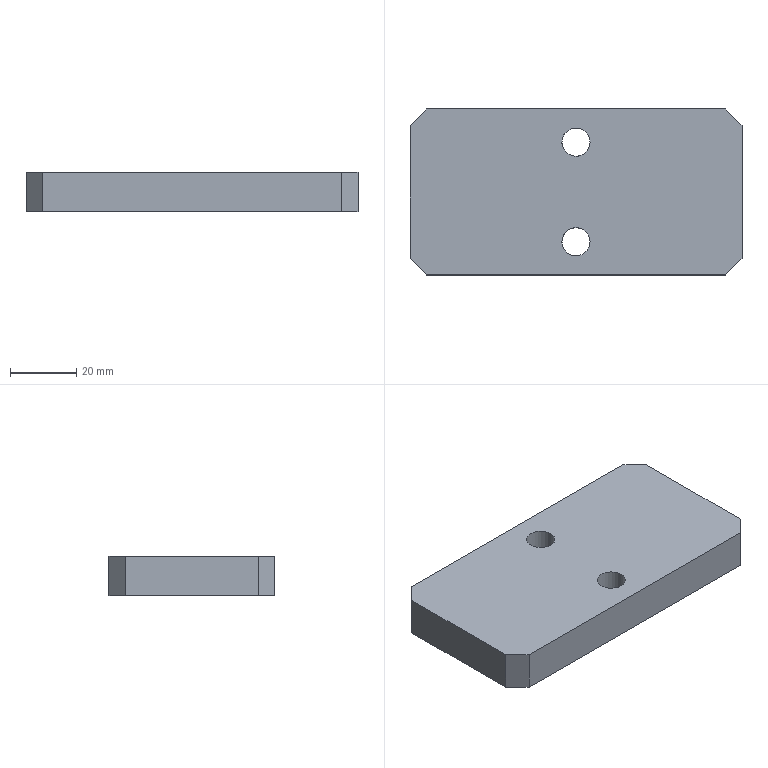Part | NX | features BREP 1 | 1 solid | 12 faces | box 100 x 50 x 12 mm | volume 58038 mm3 | plane 10 | cylinder 2 | commonest cylinder face diameters 8.5 x2
STEP:
#1=CARTESIAN_POINT('',(50.,-20.,12.));
#2=VERTEX_POINT('',#1);
#3=CARTESIAN_POINT('',(50.,20.,12.));
#4=VERTEX_POINT('',#3);
#5=CARTESIAN_POINT('',(50.,25.,12.));
#6=DIRECTION('',(0.,1.,0.));
#7=VECTOR('',#6,1000.);
#8=LINE('',#5,#7);
#9=EDGE_CURVE('',#2,#4,#8,.T.);
#10=ORIENTED_EDGE('',*,*,#9,.F.);
#11=CARTESIAN_POINT('',(50.,-20.,0.));
#12=VERTEX_POINT('',#11);
#13=CARTESIAN_POINT('',(50.,-20.,15.));
#14=DIRECTION('',(0.,0.,-1.));
#15=VECTOR('',#14,1000.);
#16=LINE('',#13,#15);
#17=EDGE_CURVE('',#2,#12,#16,.T.);
#18=ORIENTED_EDGE('',*,*,#17,.T.);
#19=CARTESIAN_POINT('',(50.,20.,0.));
#20=VERTEX_POINT('',#19);
#21=CARTESIAN_POINT('',(50.,25.,0.));
#22=DIRECTION('',(0.,1.,0.));
#23=VECTOR('',#22,1000.);
#24=LINE('',#21,#23);
#25=EDGE_CURVE('',#12,#20,#24,.T.);
#26=ORIENTED_EDGE('',*,*,#25,.T.);
#27=CARTESIAN_POINT('',(50.,20.,15.));
#28=DIRECTION('',(0.,0.,1.));
#29=VECTOR('',#28,1000.);
#30=LINE('',#27,#29);
#31=EDGE_CURVE('',#20,#4,#30,.T.);
#32=ORIENTED_EDGE('',*,*,#31,.T.);
#33=EDGE_LOOP('',(#10,#18,#26,#32));
#34=FACE_BOUND('',#33,.T.);
#35=CARTESIAN_POINT('',(50.,25.,15.));
#36=DIRECTION('',(-1.,0.,0.));
#37=DIRECTION('',(0.,0.,-1.));
#38=AXIS2_PLACEMENT_3D('',#35,#36,#37);
#39=PLANE('',#38);
#40=ADVANCED_FACE('',(#34),#39,.F.);
#41=CARTESIAN_POINT('',(45.,25.,12.));
#42=VERTEX_POINT('',#41);
#43=CARTESIAN_POINT('',(-45.,25.,12.));
#44=VERTEX_POINT('',#43);
#45=CARTESIAN_POINT('',(-50.,25.,12.));
#46=DIRECTION('',(-1.,0.,0.));
#47=VECTOR('',#46,1000.);
#48=LINE('',#45,#47);
#49=EDGE_CURVE('',#42,#44,#48,.T.);
#50=ORIENTED_EDGE('',*,*,#49,.F.);
#51=CARTESIAN_POINT('',(45.,25.,0.));
#52=VERTEX_POINT('',#51);
#53=CARTESIAN_POINT('',(45.,25.,15.));
#54=DIRECTION('',(0.,0.,-1.));
#55=VECTOR('',#54,1000.);
#56=LINE('',#53,#55);
#57=EDGE_CURVE('',#42,#52,#56,.T.);
#58=ORIENTED_EDGE('',*,*,#57,.T.);
#59=CARTESIAN_POINT('',(-45.,25.,0.));
#60=VERTEX_POINT('',#59);
#61=CARTESIAN_POINT('',(-50.,25.,0.));
#62=DIRECTION('',(-1.,0.,0.));
#63=VECTOR('',#62,1000.);
#64=LINE('',#61,#63);
#65=EDGE_CURVE('',#52,#60,#64,.T.);
#66=ORIENTED_EDGE('',*,*,#65,.T.);
#67=CARTESIAN_POINT('',(-45.,25.,15.));
#68=DIRECTION('',(0.,0.,1.));
#69=VECTOR('',#68,1000.);
#70=LINE('',#67,#69);
#71=EDGE_CURVE('',#60,#44,#70,.T.);
#72=ORIENTED_EDGE('',*,*,#71,.T.);
#73=EDGE_LOOP('',(#50,#58,#66,#72));
#74=FACE_BOUND('',#73,.T.);
#75=CARTESIAN_POINT('',(-50.,25.,15.));
#76=DIRECTION('',(0.,-1.,0.));
#77=DIRECTION('',(0.,0.,1.));
#78=AXIS2_PLACEMENT_3D('',#75,#76,#77);
#79=PLANE('',#78);
#80=ADVANCED_FACE('',(#74),#79,.F.);
#81=CARTESIAN_POINT('',(-50.,20.,12.));
#82=VERTEX_POINT('',#81);
#83=CARTESIAN_POINT('',(-50.,-20.,12.));
#84=VERTEX_POINT('',#83);
#85=CARTESIAN_POINT('',(-50.,25.,12.));
#86=DIRECTION('',(0.,-1.,0.));
#87=VECTOR('',#86,1000.);
#88=LINE('',#85,#87);
#89=EDGE_CURVE('',#82,#84,#88,.T.);
#90=ORIENTED_EDGE('',*,*,#89,.F.);
#91=CARTESIAN_POINT('',(-50.,20.,0.));
#92=VERTEX_POINT('',#91);
#93=CARTESIAN_POINT('',(-50.,20.,15.));
#94=DIRECTION('',(0.,0.,-1.));
#95=VECTOR('',#94,1000.);
#96=LINE('',#93,#95);
#97=EDGE_CURVE('',#82,#92,#96,.T.);
#98=ORIENTED_EDGE('',*,*,#97,.T.);
#99=CARTESIAN_POINT('',(-50.,-20.,0.));
#100=VERTEX_POINT('',#99);
#101=CARTESIAN_POINT('',(-50.,25.,0.));
#102=DIRECTION('',(0.,-1.,0.));
#103=VECTOR('',#102,1000.);
#104=LINE('',#101,#103);
#105=EDGE_CURVE('',#92,#100,#104,.T.);
#106=ORIENTED_EDGE('',*,*,#105,.T.);
#107=CARTESIAN_POINT('',(-50.,-20.,15.));
#108=DIRECTION('',(0.,0.,1.));
#109=VECTOR('',#108,1000.);
#110=LINE('',#107,#109);
#111=EDGE_CURVE('',#100,#84,#110,.T.);
#112=ORIENTED_EDGE('',*,*,#111,.T.);
#113=EDGE_LOOP('',(#90,#98,#106,#112));
#114=FACE_BOUND('',#113,.T.);
#115=CARTESIAN_POINT('',(-50.,25.,15.));
#116=DIRECTION('',(1.,0.,0.));
#117=DIRECTION('',(0.,0.,1.));
#118=AXIS2_PLACEMENT_3D('',#115,#116,#117);
#119=PLANE('',#118);
#120=ADVANCED_FACE('',(#114),#119,.F.);
#121=CARTESIAN_POINT('',(-45.,-25.,12.));
#122=VERTEX_POINT('',#121);
#123=CARTESIAN_POINT('',(45.,-25.,12.));
#124=VERTEX_POINT('',#123);
#125=CARTESIAN_POINT('',(-50.,-25.,12.));
#126=DIRECTION('',(1.,0.,0.));
#127=VECTOR('',#126,1000.);
#128=LINE('',#125,#127);
#129=EDGE_CURVE('',#122,#124,#128,.T.);
#130=ORIENTED_EDGE('',*,*,#129,.F.);
#131=CARTESIAN_POINT('',(-45.,-25.,0.));
#132=VERTEX_POINT('',#131);
#133=CARTESIAN_POINT('',(-45.,-25.,15.));
#134=DIRECTION('',(0.,0.,-1.));
#135=VECTOR('',#134,1000.);
#136=LINE('',#133,#135);
#137=EDGE_CURVE('',#122,#132,#136,.T.);
#138=ORIENTED_EDGE('',*,*,#137,.T.);
#139=CARTESIAN_POINT('',(45.,-25.,0.));
#140=VERTEX_POINT('',#139);
#141=CARTESIAN_POINT('',(-50.,-25.,0.));
#142=DIRECTION('',(1.,0.,0.));
#143=VECTOR('',#142,1000.);
#144=LINE('',#141,#143);
#145=EDGE_CURVE('',#132,#140,#144,.T.);
#146=ORIENTED_EDGE('',*,*,#145,.T.);
#147=CARTESIAN_POINT('',(45.,-25.,15.));
#148=DIRECTION('',(0.,0.,1.));
#149=VECTOR('',#148,1000.);
#150=LINE('',#147,#149);
#151=EDGE_CURVE('',#140,#124,#150,.T.);
#152=ORIENTED_EDGE('',*,*,#151,.T.);
#153=EDGE_LOOP('',(#130,#138,#146,#152));
#154=FACE_BOUND('',#153,.T.);
#155=CARTESIAN_POINT('',(-50.,-25.,15.));
#156=DIRECTION('',(0.,1.,0.));
#157=DIRECTION('',(0.,0.,-1.));
#158=AXIS2_PLACEMENT_3D('',#155,#156,#157);
#159=PLANE('',#158);
#160=ADVANCED_FACE('',(#154),#159,.F.);
#161=ORIENTED_EDGE('',*,*,#137,.F.);
#162=CARTESIAN_POINT('',(-45.,-25.,12.));
#163=DIRECTION('',(-0.7071,0.7071,0.));
#164=VECTOR('',#163,1000.);
#165=LINE('',#162,#164);
#166=EDGE_CURVE('',#122,#84,#165,.T.);
#167=ORIENTED_EDGE('',*,*,#166,.T.);
#168=ORIENTED_EDGE('',*,*,#111,.F.);
#169=CARTESIAN_POINT('',(-45.,-25.,0.));
#170=DIRECTION('',(-0.7071,0.7071,0.));
#171=VECTOR('',#170,1000.);
#172=LINE('',#169,#171);
#173=EDGE_CURVE('',#132,#100,#172,.T.);
#174=ORIENTED_EDGE('',*,*,#173,.F.);
#175=EDGE_LOOP('',(#161,#167,#168,#174));
#176=FACE_BOUND('',#175,.T.);
#177=CARTESIAN_POINT('',(-45.,-25.,15.));
#178=DIRECTION('',(0.7071,0.7071,0.));
#179=DIRECTION('',(0.,0.,1.));
#180=AXIS2_PLACEMENT_3D('',#177,#178,#179);
#181=PLANE('',#180);
#182=ADVANCED_FACE('',(#176),#181,.F.);
#183=ORIENTED_EDGE('',*,*,#97,.F.);
#184=CARTESIAN_POINT('',(-50.,20.,12.));
#185=DIRECTION('',(0.7071,0.7071,0.));
#186=VECTOR('',#185,1000.);
#187=LINE('',#184,#186);
#188=EDGE_CURVE('',#82,#44,#187,.T.);
#189=ORIENTED_EDGE('',*,*,#188,.T.);
#190=ORIENTED_EDGE('',*,*,#71,.F.);
#191=CARTESIAN_POINT('',(-50.,20.,0.));
#192=DIRECTION('',(0.7071,0.7071,0.));
#193=VECTOR('',#192,1000.);
#194=LINE('',#191,#193);
#195=EDGE_CURVE('',#92,#60,#194,.T.);
#196=ORIENTED_EDGE('',*,*,#195,.F.);
#197=EDGE_LOOP('',(#183,#189,#190,#196));
#198=FACE_BOUND('',#197,.T.);
#199=CARTESIAN_POINT('',(-50.,20.,15.));
#200=DIRECTION('',(0.7071,-0.7071,0.));
#201=DIRECTION('',(0.,0.,1.));
#202=AXIS2_PLACEMENT_3D('',#199,#200,#201);
#203=PLANE('',#202);
#204=ADVANCED_FACE('',(#198),#203,.F.);
#205=ORIENTED_EDGE('',*,*,#17,.F.);
#206=CARTESIAN_POINT('',(50.,-20.,12.));
#207=DIRECTION('',(-0.7071,-0.7071,0.));
#208=VECTOR('',#207,1000.);
#209=LINE('',#206,#208);
#210=EDGE_CURVE('',#2,#124,#209,.T.);
#211=ORIENTED_EDGE('',*,*,#210,.T.);
#212=ORIENTED_EDGE('',*,*,#151,.F.);
#213=CARTESIAN_POINT('',(50.,-20.,0.));
#214=DIRECTION('',(-0.7071,-0.7071,0.));
#215=VECTOR('',#214,1000.);
#216=LINE('',#213,#215);
#217=EDGE_CURVE('',#12,#140,#216,.T.);
#218=ORIENTED_EDGE('',*,*,#217,.F.);
#219=EDGE_LOOP('',(#205,#211,#212,#218));
#220=FACE_BOUND('',#219,.T.);
#221=CARTESIAN_POINT('',(50.,-20.,15.));
#222=DIRECTION('',(-0.7071,0.7071,0.));
#223=DIRECTION('',(0.,0.,1.));
#224=AXIS2_PLACEMENT_3D('',#221,#222,#223);
#225=PLANE('',#224);
#226=ADVANCED_FACE('',(#220),#225,.F.);
#227=ORIENTED_EDGE('',*,*,#57,.F.);
#228=CARTESIAN_POINT('',(45.,25.,12.));
#229=DIRECTION('',(0.7071,-0.7071,0.));
#230=VECTOR('',#229,1000.);
#231=LINE('',#228,#230);
#232=EDGE_CURVE('',#42,#4,#231,.T.);
#233=ORIENTED_EDGE('',*,*,#232,.T.);
#234=ORIENTED_EDGE('',*,*,#31,.F.);
#235=CARTESIAN_POINT('',(45.,25.,0.));
#236=DIRECTION('',(0.7071,-0.7071,0.));
#237=VECTOR('',#236,1000.);
#238=LINE('',#235,#237);
#239=EDGE_CURVE('',#52,#20,#238,.T.);
#240=ORIENTED_EDGE('',*,*,#239,.F.);
#241=EDGE_LOOP('',(#227,#233,#234,#240));
#242=FACE_BOUND('',#241,.T.);
#243=CARTESIAN_POINT('',(45.,25.,15.));
#244=DIRECTION('',(-0.7071,-0.7071,0.));
#245=DIRECTION('',(0.,0.,1.));
#246=AXIS2_PLACEMENT_3D('',#243,#244,#245);
#247=PLANE('',#246);
#248=ADVANCED_FACE('',(#242),#247,.F.);
#249=CARTESIAN_POINT('',(4.25,15.,0.));
#250=VERTEX_POINT('',#249);
#251=CARTESIAN_POINT('',(0.,15.,0.));
#252=DIRECTION('',(0.,0.,1.));
#253=DIRECTION('',(1.,0.,0.));
#254=AXIS2_PLACEMENT_3D('',#251,#252,#253);
#255=CIRCLE('',#254,4.25);
#256=EDGE_CURVE('',#250,#250,#255,.T.);
#257=ORIENTED_EDGE('',*,*,#256,.T.);
#258=EDGE_LOOP('',(#257));
#259=FACE_BOUND('',#258,.T.);
#260=CARTESIAN_POINT('',(4.25,-15.,0.));
#261=VERTEX_POINT('',#260);
#262=CARTESIAN_POINT('',(0.,-15.,0.));
#263=DIRECTION('',(0.,0.,1.));
#264=DIRECTION('',(1.,0.,0.));
#265=AXIS2_PLACEMENT_3D('',#262,#263,#264);
#266=CIRCLE('',#265,4.25);
#267=EDGE_CURVE('',#261,#261,#266,.T.);
#268=ORIENTED_EDGE('',*,*,#267,.T.);
#269=EDGE_LOOP('',(#268));
#270=FACE_BOUND('',#269,.T.);
#271=ORIENTED_EDGE('',*,*,#145,.F.);
#272=ORIENTED_EDGE('',*,*,#173,.T.);
#273=ORIENTED_EDGE('',*,*,#105,.F.);
#274=ORIENTED_EDGE('',*,*,#195,.T.);
#275=ORIENTED_EDGE('',*,*,#65,.F.);
#276=ORIENTED_EDGE('',*,*,#239,.T.);
#277=ORIENTED_EDGE('',*,*,#25,.F.);
#278=ORIENTED_EDGE('',*,*,#217,.T.);
#279=EDGE_LOOP('',(#271,#272,#273,#274,#275,#276,#277,#278));
#280=FACE_BOUND('',#279,.T.);
#281=CARTESIAN_POINT('',(0.,0.,0.));
#282=DIRECTION('',(0.,0.,1.));
#283=DIRECTION('',(-1.,0.,0.));
#284=AXIS2_PLACEMENT_3D('',#281,#282,#283);
#285=PLANE('',#284);
#286=ADVANCED_FACE('',(#259,#270,#280),#285,.F.);
#287=CARTESIAN_POINT('',(0.,10.75,12.));
#288=VERTEX_POINT('',#287);
#289=CARTESIAN_POINT('',(0.,15.,12.));
#290=DIRECTION('',(0.,0.,1.));
#291=DIRECTION('',(0.,-1.,0.));
#292=AXIS2_PLACEMENT_3D('',#289,#290,#291);
#293=CIRCLE('',#292,4.25);
#294=EDGE_CURVE('',#288,#288,#293,.T.);
#295=ORIENTED_EDGE('',*,*,#294,.F.);
#296=EDGE_LOOP('',(#295));
#297=FACE_BOUND('',#296,.T.);
#298=CARTESIAN_POINT('',(0.,-19.25,12.));
#299=VERTEX_POINT('',#298);
#300=CARTESIAN_POINT('',(0.,-15.,12.));
#301=DIRECTION('',(0.,0.,1.));
#302=DIRECTION('',(0.,-1.,0.));
#303=AXIS2_PLACEMENT_3D('',#300,#301,#302);
#304=CIRCLE('',#303,4.25);
#305=EDGE_CURVE('',#299,#299,#304,.T.);
#306=ORIENTED_EDGE('',*,*,#305,.F.);
#307=EDGE_LOOP('',(#306));
#308=FACE_BOUND('',#307,.T.);
#309=ORIENTED_EDGE('',*,*,#129,.T.);
#310=ORIENTED_EDGE('',*,*,#210,.F.);
#311=ORIENTED_EDGE('',*,*,#9,.T.);
#312=ORIENTED_EDGE('',*,*,#232,.F.);
#313=ORIENTED_EDGE('',*,*,#49,.T.);
#314=ORIENTED_EDGE('',*,*,#188,.F.);
#315=ORIENTED_EDGE('',*,*,#89,.T.);
#316=ORIENTED_EDGE('',*,*,#166,.F.);
#317=EDGE_LOOP('',(#309,#310,#311,#312,#313,#314,#315,#316));
#318=FACE_BOUND('',#317,.T.);
#319=CARTESIAN_POINT('',(-25.,-380.,12.));
#320=DIRECTION('',(0.,0.,1.));
#321=DIRECTION('',(0.,1.,0.));
#322=AXIS2_PLACEMENT_3D('',#319,#320,#321);
#323=PLANE('',#322);
#324=ADVANCED_FACE('',(#297,#308,#318),#323,.T.);
#325=ORIENTED_EDGE('',*,*,#305,.T.);
#326=EDGE_LOOP('',(#325));
#327=FACE_BOUND('',#326,.T.);
#328=ORIENTED_EDGE('',*,*,#267,.F.);
#329=EDGE_LOOP('',(#328));
#330=FACE_BOUND('',#329,.T.);
#331=CARTESIAN_POINT('',(0.,-15.,12.));
#332=DIRECTION('',(0.,0.,1.));
#333=DIRECTION('',(0.,1.,0.));
#334=AXIS2_PLACEMENT_3D('',#331,#332,#333);
#335=CYLINDRICAL_SURFACE('',#334,4.25);
#336=ADVANCED_FACE('',(#327,#330),#335,.F.);
#337=ORIENTED_EDGE('',*,*,#294,.T.);
#338=EDGE_LOOP('',(#337));
#339=FACE_BOUND('',#338,.T.);
#340=ORIENTED_EDGE('',*,*,#256,.F.);
#341=EDGE_LOOP('',(#340));
#342=FACE_BOUND('',#341,.T.);
#343=CARTESIAN_POINT('',(0.,15.,12.));
#344=DIRECTION('',(0.,0.,1.));
#345=DIRECTION('',(0.,1.,0.));
#346=AXIS2_PLACEMENT_3D('',#343,#344,#345);
#347=CYLINDRICAL_SURFACE('',#346,4.25);
#348=ADVANCED_FACE('',(#339,#342),#347,.F.);
#349=CLOSED_SHELL('',(#40,#80,#120,#160,#182,#204,#226,#248,#286,#324,#336,#348));
#350=MANIFOLD_SOLID_BREP('',#349);
#351=(LENGTH_UNIT()NAMED_UNIT(*)SI_UNIT(.MILLI.,.METRE.));
#352=UNCERTAINTY_MEASURE_WITH_UNIT(LENGTH_MEASURE(0.00001),#351,'','');
#353=(NAMED_UNIT(*)PLANE_ANGLE_UNIT()SI_UNIT($,.RADIAN.));
#354=(NAMED_UNIT(*)SI_UNIT($,.STERADIAN.)SOLID_ANGLE_UNIT());
#355=(GEOMETRIC_REPRESENTATION_CONTEXT(3)GLOBAL_UNCERTAINTY_ASSIGNED_CONTEXT((#352))GLOBAL_UNIT_ASSIGNED_CONTEXT((#351,#353,#354))REPRESENTATION_CONTEXT('',''));
#356=ADVANCED_BREP_SHAPE_REPRESENTATION('',(#350),#355);